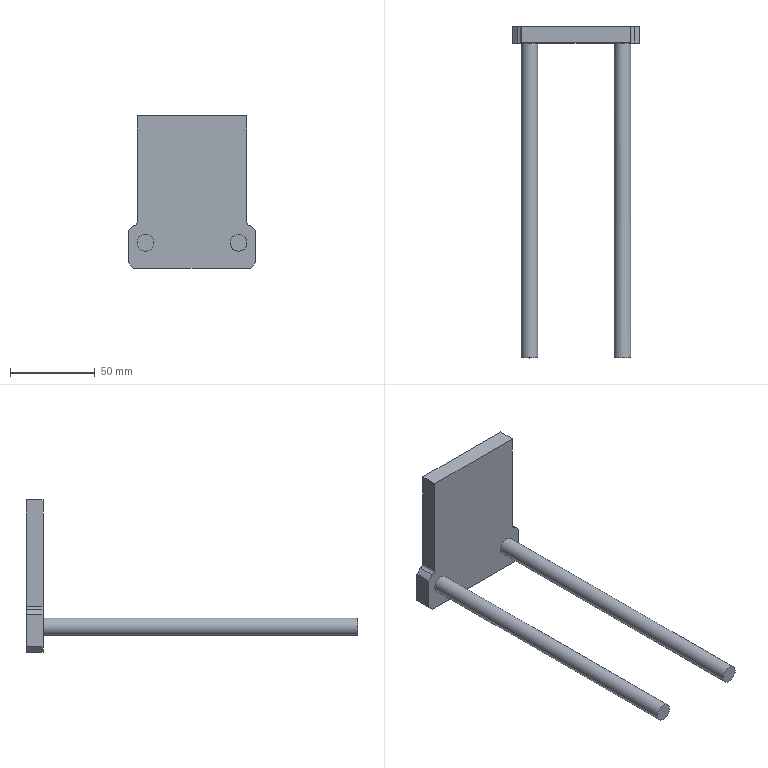Part | STEP file | Tube necking machine_id406_x_t | 1 solid | 18 faces | box 75 x 196.3 x 90 mm | volume 90101 mm3 | plane 14 | cylinder 4 | commonest cylinder face diameters 4 x2 10 x2
STEP:
#1=CARTESIAN_POINT('',(0.,0.,0.));
#2=DIRECTION('',(0.,0.,1.));
#3=DIRECTION('',(1.,0.,0.));
#4=AXIS2_PLACEMENT_3D('',#1,#2,#3);
#5=CARTESIAN_POINT('',(-32.452,292.8,213.016));
#6=VERTEX_POINT('',#5);
#7=CARTESIAN_POINT('',(-32.452,292.8,276.016));
#8=VERTEX_POINT('',#7);
#9=CARTESIAN_POINT('',(-32.452,292.8,186.016));
#10=DIRECTION('',(0.,0.,1.));
#11=VECTOR('',#10,1.);
#12=LINE('',#9,#11);
#13=CARTESIAN_POINT('',(-32.452,292.8,186.016));
#14=DIRECTION('',(1.,0.,0.));
#15=DIRECTION('',(0.,0.,-1.));
#16=AXIS2_PLACEMENT_3D('',#13,#14,#15);
#17=PLANE('',#16);
#18=CARTESIAN_POINT('',(0.,0.));
#19=DIRECTION('',(-1.,0.));
#20=VECTOR('',#19,1.);
#21=LINE('',#18,#20);
#22=(GEOMETRIC_REPRESENTATION_CONTEXT(2)PARAMETRIC_REPRESENTATION_CONTEXT()REPRESENTATION_CONTEXT('',''));
#23=DEFINITIONAL_REPRESENTATION('',(#21),#22);
#24=PCURVE('',#17,#23);
#25=CARTESIAN_POINT('',(0.,292.8,25.));
#26=DIRECTION('',(0.,1.,0.));
#27=DIRECTION('',(0.,0.,1.));
#28=AXIS2_PLACEMENT_3D('',#25,#26,#27);
#29=PLANE('',#28);
#30=CARTESIAN_POINT('',(161.016,-32.452));
#31=DIRECTION('',(1.,0.));
#32=VECTOR('',#31,1.);
#33=LINE('',#30,#32);
#34=(GEOMETRIC_REPRESENTATION_CONTEXT(2)PARAMETRIC_REPRESENTATION_CONTEXT()REPRESENTATION_CONTEXT('',''));
#35=DEFINITIONAL_REPRESENTATION('',(#33),#34);
#36=PCURVE('',#29,#35);
#37=SURFACE_CURVE('',#12,(#24,#36),.PCURVE_S1.);
#38=EDGE_CURVE('',#6,#8,#37,.T.);
#39=ORIENTED_EDGE('',*,*,#38,.F.);
#40=CARTESIAN_POINT('',(-32.452,282.8,213.016));
#41=VERTEX_POINT('',#40);
#42=CARTESIAN_POINT('',(-32.452,292.8,213.016));
#43=DIRECTION('',(0.,-1.,0.));
#44=VECTOR('',#43,1.);
#45=LINE('',#42,#44);
#46=CARTESIAN_POINT('',(-27.,0.));
#47=DIRECTION('',(0.,-1.));
#48=VECTOR('',#47,1.);
#49=LINE('',#46,#48);
#50=(GEOMETRIC_REPRESENTATION_CONTEXT(2)PARAMETRIC_REPRESENTATION_CONTEXT()REPRESENTATION_CONTEXT('',''));
#51=DEFINITIONAL_REPRESENTATION('',(#49),#50);
#52=PCURVE('',#17,#51);
#53=CARTESIAN_POINT('',(-34.452,282.8,213.016));
#54=DIRECTION('',(0.,1.,0.));
#55=DIRECTION('',(0.,0.,1.));
#56=AXIS2_PLACEMENT_3D('',#53,#54,#55);
#57=CYLINDRICAL_SURFACE('',#56,2.);
#58=CARTESIAN_POINT('',(1.571,10.));
#59=DIRECTION('',(0.,-1.));
#60=VECTOR('',#59,1.);
#61=LINE('',#58,#60);
#62=(GEOMETRIC_REPRESENTATION_CONTEXT(2)PARAMETRIC_REPRESENTATION_CONTEXT()REPRESENTATION_CONTEXT('',''));
#63=DEFINITIONAL_REPRESENTATION('',(#61),#62);
#64=PCURVE('',#57,#63);
#65=SURFACE_CURVE('',#45,(#52,#64),.PCURVE_S1.);
#66=EDGE_CURVE('',#6,#41,#65,.T.);
#67=ORIENTED_EDGE('',*,*,#66,.T.);
#68=CARTESIAN_POINT('',(-32.452,282.8,276.016));
#69=VERTEX_POINT('',#68);
#70=CARTESIAN_POINT('',(-32.452,282.8,186.016));
#71=DIRECTION('',(0.,0.,1.));
#72=VECTOR('',#71,1.);
#73=LINE('',#70,#72);
#74=CARTESIAN_POINT('',(0.,-10.));
#75=DIRECTION('',(-1.,0.));
#76=VECTOR('',#75,1.);
#77=LINE('',#74,#76);
#78=(GEOMETRIC_REPRESENTATION_CONTEXT(2)PARAMETRIC_REPRESENTATION_CONTEXT()REPRESENTATION_CONTEXT('',''));
#79=DEFINITIONAL_REPRESENTATION('',(#77),#78);
#80=PCURVE('',#17,#79);
#81=CARTESIAN_POINT('',(0.,282.8,25.));
#82=DIRECTION('',(0.,1.,0.));
#83=DIRECTION('',(0.,0.,1.));
#84=AXIS2_PLACEMENT_3D('',#81,#82,#83);
#85=PLANE('',#84);
#86=CARTESIAN_POINT('',(161.016,-32.452));
#87=DIRECTION('',(1.,0.));
#88=VECTOR('',#87,1.);
#89=LINE('',#86,#88);
#90=(GEOMETRIC_REPRESENTATION_CONTEXT(2)PARAMETRIC_REPRESENTATION_CONTEXT()REPRESENTATION_CONTEXT('',''));
#91=DEFINITIONAL_REPRESENTATION('',(#89),#90);
#92=PCURVE('',#85,#91);
#93=SURFACE_CURVE('',#73,(#80,#92),.PCURVE_S1.);
#94=EDGE_CURVE('',#41,#69,#93,.T.);
#95=ORIENTED_EDGE('',*,*,#94,.T.);
#96=CARTESIAN_POINT('',(-32.452,292.8,276.016));
#97=DIRECTION('',(0.,-1.,0.));
#98=VECTOR('',#97,1.);
#99=LINE('',#96,#98);
#100=CARTESIAN_POINT('',(-90.,0.));
#101=DIRECTION('',(0.,-1.));
#102=VECTOR('',#101,1.);
#103=LINE('',#100,#102);
#104=(GEOMETRIC_REPRESENTATION_CONTEXT(2)PARAMETRIC_REPRESENTATION_CONTEXT()REPRESENTATION_CONTEXT('',''));
#105=DEFINITIONAL_REPRESENTATION('',(#103),#104);
#106=PCURVE('',#17,#105);
#107=CARTESIAN_POINT('',(-32.452,292.8,276.016));
#108=DIRECTION('',(0.,0.,-1.));
#109=DIRECTION('',(-1.,0.,0.));
#110=AXIS2_PLACEMENT_3D('',#107,#108,#109);
#111=PLANE('',#110);
#112=CARTESIAN_POINT('',(0.,0.));
#113=DIRECTION('',(0.,-1.));
#114=VECTOR('',#113,1.);
#115=LINE('',#112,#114);
#116=(GEOMETRIC_REPRESENTATION_CONTEXT(2)PARAMETRIC_REPRESENTATION_CONTEXT()REPRESENTATION_CONTEXT('',''));
#117=DEFINITIONAL_REPRESENTATION('',(#115),#116);
#118=PCURVE('',#111,#117);
#119=SURFACE_CURVE('',#99,(#106,#118),.PCURVE_S1.);
#120=EDGE_CURVE('',#8,#69,#119,.T.);
#121=ORIENTED_EDGE('',*,*,#120,.F.);
#122=EDGE_LOOP('',(#39,#67,#95,#121));
#123=FACE_BOUND('',#122,.T.);
#124=ADVANCED_FACE('',(#123),#17,.F.);
#125=CARTESIAN_POINT('',(32.548,282.8,276.016));
#126=VERTEX_POINT('',#125);
#127=CARTESIAN_POINT('',(-32.452,282.8,276.016));
#128=DIRECTION('',(1.,0.,0.));
#129=VECTOR('',#128,1.);
#130=LINE('',#127,#129);
#131=CARTESIAN_POINT('',(0.,-10.));
#132=DIRECTION('',(-1.,0.));
#133=VECTOR('',#132,1.);
#134=LINE('',#131,#133);
#135=(GEOMETRIC_REPRESENTATION_CONTEXT(2)PARAMETRIC_REPRESENTATION_CONTEXT()REPRESENTATION_CONTEXT('',''));
#136=DEFINITIONAL_REPRESENTATION('',(#134),#135);
#137=PCURVE('',#111,#136);
#138=CARTESIAN_POINT('',(251.016,-32.452));
#139=DIRECTION('',(0.,1.));
#140=VECTOR('',#139,1.);
#141=LINE('',#138,#140);
#142=(GEOMETRIC_REPRESENTATION_CONTEXT(2)PARAMETRIC_REPRESENTATION_CONTEXT()REPRESENTATION_CONTEXT('',''));
#143=DEFINITIONAL_REPRESENTATION('',(#141),#142);
#144=PCURVE('',#85,#143);
#145=SURFACE_CURVE('',#130,(#137,#144),.PCURVE_S1.);
#146=EDGE_CURVE('',#69,#126,#145,.T.);
#147=ORIENTED_EDGE('',*,*,#146,.T.);
#148=CARTESIAN_POINT('',(32.548,292.8,276.016));
#149=VERTEX_POINT('',#148);
#150=CARTESIAN_POINT('',(32.548,292.8,276.016));
#151=DIRECTION('',(0.,-1.,0.));
#152=VECTOR('',#151,1.);
#153=LINE('',#150,#152);
#154=CARTESIAN_POINT('',(-65.,0.));
#155=DIRECTION('',(0.,-1.));
#156=VECTOR('',#155,1.);
#157=LINE('',#154,#156);
#158=(GEOMETRIC_REPRESENTATION_CONTEXT(2)PARAMETRIC_REPRESENTATION_CONTEXT()REPRESENTATION_CONTEXT('',''));
#159=DEFINITIONAL_REPRESENTATION('',(#157),#158);
#160=PCURVE('',#111,#159);
#161=CARTESIAN_POINT('',(32.548,292.8,276.016));
#162=DIRECTION('',(-1.,0.,0.));
#163=DIRECTION('',(0.,0.,1.));
#164=AXIS2_PLACEMENT_3D('',#161,#162,#163);
#165=PLANE('',#164);
#166=CARTESIAN_POINT('',(0.,0.));
#167=DIRECTION('',(0.,-1.));
#168=VECTOR('',#167,1.);
#169=LINE('',#166,#168);
#170=(GEOMETRIC_REPRESENTATION_CONTEXT(2)PARAMETRIC_REPRESENTATION_CONTEXT()REPRESENTATION_CONTEXT('',''));
#171=DEFINITIONAL_REPRESENTATION('',(#169),#170);
#172=PCURVE('',#165,#171);
#173=SURFACE_CURVE('',#153,(#160,#172),.PCURVE_S1.);
#174=EDGE_CURVE('',#149,#126,#173,.T.);
#175=ORIENTED_EDGE('',*,*,#174,.F.);
#176=CARTESIAN_POINT('',(-32.452,292.8,276.016));
#177=DIRECTION('',(1.,0.,0.));
#178=VECTOR('',#177,1.);
#179=LINE('',#176,#178);
#180=CARTESIAN_POINT('',(0.,0.));
#181=DIRECTION('',(-1.,0.));
#182=VECTOR('',#181,1.);
#183=LINE('',#180,#182);
#184=(GEOMETRIC_REPRESENTATION_CONTEXT(2)PARAMETRIC_REPRESENTATION_CONTEXT()REPRESENTATION_CONTEXT('',''));
#185=DEFINITIONAL_REPRESENTATION('',(#183),#184);
#186=PCURVE('',#111,#185);
#187=CARTESIAN_POINT('',(251.016,-32.452));
#188=DIRECTION('',(0.,1.));
#189=VECTOR('',#188,1.);
#190=LINE('',#187,#189);
#191=(GEOMETRIC_REPRESENTATION_CONTEXT(2)PARAMETRIC_REPRESENTATION_CONTEXT()REPRESENTATION_CONTEXT('',''));
#192=DEFINITIONAL_REPRESENTATION('',(#190),#191);
#193=PCURVE('',#29,#192);
#194=SURFACE_CURVE('',#179,(#186,#193),.PCURVE_S1.);
#195=EDGE_CURVE('',#8,#149,#194,.T.);
#196=ORIENTED_EDGE('',*,*,#195,.F.);
#197=ORIENTED_EDGE('',*,*,#120,.T.);
#198=EDGE_LOOP('',(#147,#175,#196,#197));
#199=FACE_BOUND('',#198,.T.);
#200=ADVANCED_FACE('',(#199),#111,.F.);
#201=CARTESIAN_POINT('',(32.548,282.8,213.016));
#202=VERTEX_POINT('',#201);
#203=CARTESIAN_POINT('',(32.548,282.8,276.016));
#204=DIRECTION('',(0.,0.,-1.));
#205=VECTOR('',#204,1.);
#206=LINE('',#203,#205);
#207=CARTESIAN_POINT('',(0.,-10.));
#208=DIRECTION('',(-1.,0.));
#209=VECTOR('',#208,1.);
#210=LINE('',#207,#209);
#211=(GEOMETRIC_REPRESENTATION_CONTEXT(2)PARAMETRIC_REPRESENTATION_CONTEXT()REPRESENTATION_CONTEXT('',''));
#212=DEFINITIONAL_REPRESENTATION('',(#210),#211);
#213=PCURVE('',#165,#212);
#214=CARTESIAN_POINT('',(251.016,32.548));
#215=DIRECTION('',(-1.,0.));
#216=VECTOR('',#215,1.);
#217=LINE('',#214,#216);
#218=(GEOMETRIC_REPRESENTATION_CONTEXT(2)PARAMETRIC_REPRESENTATION_CONTEXT()REPRESENTATION_CONTEXT('',''));
#219=DEFINITIONAL_REPRESENTATION('',(#217),#218);
#220=PCURVE('',#85,#219);
#221=SURFACE_CURVE('',#206,(#213,#220),.PCURVE_S1.);
#222=EDGE_CURVE('',#126,#202,#221,.T.);
#223=ORIENTED_EDGE('',*,*,#222,.T.);
#224=CARTESIAN_POINT('',(32.548,292.8,213.016));
#225=VERTEX_POINT('',#224);
#226=CARTESIAN_POINT('',(32.548,292.8,213.016));
#227=DIRECTION('',(0.,1.,0.));
#228=VECTOR('',#227,1.);
#229=LINE('',#226,#228);
#230=CARTESIAN_POINT('',(-63.,0.));
#231=DIRECTION('',(0.,1.));
#232=VECTOR('',#231,1.);
#233=LINE('',#230,#232);
#234=(GEOMETRIC_REPRESENTATION_CONTEXT(2)PARAMETRIC_REPRESENTATION_CONTEXT()REPRESENTATION_CONTEXT('',''));
#235=DEFINITIONAL_REPRESENTATION('',(#233),#234);
#236=PCURVE('',#165,#235);
#237=CARTESIAN_POINT('',(34.548,292.8,213.016));
#238=DIRECTION('',(0.,-1.,0.));
#239=DIRECTION('',(0.,0.,-1.));
#240=AXIS2_PLACEMENT_3D('',#237,#238,#239);
#241=CYLINDRICAL_SURFACE('',#240,2.);
#242=CARTESIAN_POINT('',(4.712,0.));
#243=DIRECTION('',(0.,-1.));
#244=VECTOR('',#243,1.);
#245=LINE('',#242,#244);
#246=(GEOMETRIC_REPRESENTATION_CONTEXT(2)PARAMETRIC_REPRESENTATION_CONTEXT()REPRESENTATION_CONTEXT('',''));
#247=DEFINITIONAL_REPRESENTATION('',(#245),#246);
#248=PCURVE('',#241,#247);
#249=SURFACE_CURVE('',#229,(#236,#248),.PCURVE_S1.);
#250=EDGE_CURVE('',#202,#225,#249,.T.);
#251=ORIENTED_EDGE('',*,*,#250,.T.);
#252=CARTESIAN_POINT('',(32.548,292.8,276.016));
#253=DIRECTION('',(0.,0.,-1.));
#254=VECTOR('',#253,1.);
#255=LINE('',#252,#254);
#256=CARTESIAN_POINT('',(0.,0.));
#257=DIRECTION('',(-1.,0.));
#258=VECTOR('',#257,1.);
#259=LINE('',#256,#258);
#260=(GEOMETRIC_REPRESENTATION_CONTEXT(2)PARAMETRIC_REPRESENTATION_CONTEXT()REPRESENTATION_CONTEXT('',''));
#261=DEFINITIONAL_REPRESENTATION('',(#259),#260);
#262=PCURVE('',#165,#261);
#263=CARTESIAN_POINT('',(251.016,32.548));
#264=DIRECTION('',(-1.,0.));
#265=VECTOR('',#264,1.);
#266=LINE('',#263,#265);
#267=(GEOMETRIC_REPRESENTATION_CONTEXT(2)PARAMETRIC_REPRESENTATION_CONTEXT()REPRESENTATION_CONTEXT('',''));
#268=DEFINITIONAL_REPRESENTATION('',(#266),#267);
#269=PCURVE('',#29,#268);
#270=SURFACE_CURVE('',#255,(#262,#269),.PCURVE_S1.);
#271=EDGE_CURVE('',#149,#225,#270,.T.);
#272=ORIENTED_EDGE('',*,*,#271,.F.);
#273=ORIENTED_EDGE('',*,*,#174,.T.);
#274=EDGE_LOOP('',(#223,#251,#272,#273));
#275=FACE_BOUND('',#274,.T.);
#276=ADVANCED_FACE('',(#275),#165,.F.);
#277=CARTESIAN_POINT('',(34.548,292.8,186.016));
#278=VERTEX_POINT('',#277);
#279=CARTESIAN_POINT('',(-34.452,292.8,186.016));
#280=VERTEX_POINT('',#279);
#281=CARTESIAN_POINT('',(32.548,292.8,186.016));
#282=DIRECTION('',(-1.,0.,0.));
#283=VECTOR('',#282,1.);
#284=LINE('',#281,#283);
#285=CARTESIAN_POINT('',(32.548,292.8,186.016));
#286=DIRECTION('',(0.,0.,1.));
#287=DIRECTION('',(1.,0.,0.));
#288=AXIS2_PLACEMENT_3D('',#285,#286,#287);
#289=PLANE('',#288);
#290=CARTESIAN_POINT('',(0.,0.));
#291=DIRECTION('',(-1.,0.));
#292=VECTOR('',#291,1.);
#293=LINE('',#290,#292);
#294=(GEOMETRIC_REPRESENTATION_CONTEXT(2)PARAMETRIC_REPRESENTATION_CONTEXT()REPRESENTATION_CONTEXT('',''));
#295=DEFINITIONAL_REPRESENTATION('',(#293),#294);
#296=PCURVE('',#289,#295);
#297=CARTESIAN_POINT('',(161.016,32.548));
#298=DIRECTION('',(0.,-1.));
#299=VECTOR('',#298,1.);
#300=LINE('',#297,#299);
#301=(GEOMETRIC_REPRESENTATION_CONTEXT(2)PARAMETRIC_REPRESENTATION_CONTEXT()REPRESENTATION_CONTEXT('',''));
#302=DEFINITIONAL_REPRESENTATION('',(#300),#301);
#303=PCURVE('',#29,#302);
#304=SURFACE_CURVE('',#284,(#296,#303),.PCURVE_S1.);
#305=EDGE_CURVE('',#278,#280,#304,.T.);
#306=ORIENTED_EDGE('',*,*,#305,.F.);
#307=CARTESIAN_POINT('',(34.548,282.8,186.016));
#308=VERTEX_POINT('',#307);
#309=CARTESIAN_POINT('',(34.548,292.8,186.016));
#310=DIRECTION('',(0.,-1.,0.));
#311=VECTOR('',#310,1.);
#312=LINE('',#309,#311);
#313=CARTESIAN_POINT('',(2.,0.));
#314=DIRECTION('',(0.,-1.));
#315=VECTOR('',#314,1.);
#316=LINE('',#313,#315);
#317=(GEOMETRIC_REPRESENTATION_CONTEXT(2)PARAMETRIC_REPRESENTATION_CONTEXT()REPRESENTATION_CONTEXT('',''));
#318=DEFINITIONAL_REPRESENTATION('',(#316),#317);
#319=PCURVE('',#289,#318);
#320=CARTESIAN_POINT('',(37.548,282.8,189.016));
#321=DIRECTION('',(-0.7071,0.,0.7071));
#322=DIRECTION('',(0.,1.,0.));
#323=AXIS2_PLACEMENT_3D('',#320,#321,#322);
#324=PLANE('',#323);
#325=CARTESIAN_POINT('',(10.,4.243));
#326=DIRECTION('',(-1.,0.));
#327=VECTOR('',#326,1.);
#328=LINE('',#325,#327);
#329=(GEOMETRIC_REPRESENTATION_CONTEXT(2)PARAMETRIC_REPRESENTATION_CONTEXT()REPRESENTATION_CONTEXT('',''));
#330=DEFINITIONAL_REPRESENTATION('',(#328),#329);
#331=PCURVE('',#324,#330);
#332=SURFACE_CURVE('',#312,(#319,#331),.PCURVE_S1.);
#333=EDGE_CURVE('',#278,#308,#332,.T.);
#334=ORIENTED_EDGE('',*,*,#333,.T.);
#335=CARTESIAN_POINT('',(-34.452,282.8,186.016));
#336=VERTEX_POINT('',#335);
#337=CARTESIAN_POINT('',(32.548,282.8,186.016));
#338=DIRECTION('',(-1.,0.,0.));
#339=VECTOR('',#338,1.);
#340=LINE('',#337,#339);
#341=CARTESIAN_POINT('',(0.,-10.));
#342=DIRECTION('',(-1.,0.));
#343=VECTOR('',#342,1.);
#344=LINE('',#341,#343);
#345=(GEOMETRIC_REPRESENTATION_CONTEXT(2)PARAMETRIC_REPRESENTATION_CONTEXT()REPRESENTATION_CONTEXT('',''));
#346=DEFINITIONAL_REPRESENTATION('',(#344),#345);
#347=PCURVE('',#289,#346);
#348=CARTESIAN_POINT('',(161.016,32.548));
#349=DIRECTION('',(0.,-1.));
#350=VECTOR('',#349,1.);
#351=LINE('',#348,#350);
#352=(GEOMETRIC_REPRESENTATION_CONTEXT(2)PARAMETRIC_REPRESENTATION_CONTEXT()REPRESENTATION_CONTEXT('',''));
#353=DEFINITIONAL_REPRESENTATION('',(#351),#352);
#354=PCURVE('',#85,#353);
#355=SURFACE_CURVE('',#340,(#347,#354),.PCURVE_S1.);
#356=EDGE_CURVE('',#308,#336,#355,.T.);
#357=ORIENTED_EDGE('',*,*,#356,.T.);
#358=CARTESIAN_POINT('',(-34.452,292.8,186.016));
#359=DIRECTION('',(0.,1.,0.));
#360=VECTOR('',#359,1.);
#361=LINE('',#358,#360);
#362=CARTESIAN_POINT('',(-67.,0.));
#363=DIRECTION('',(0.,1.));
#364=VECTOR('',#363,1.);
#365=LINE('',#362,#364);
#366=(GEOMETRIC_REPRESENTATION_CONTEXT(2)PARAMETRIC_REPRESENTATION_CONTEXT()REPRESENTATION_CONTEXT('',''));
#367=DEFINITIONAL_REPRESENTATION('',(#365),#366);
#368=PCURVE('',#289,#367);
#369=CARTESIAN_POINT('',(-34.452,292.8,186.016));
#370=DIRECTION('',(-0.7071,0.,-0.7071));
#371=DIRECTION('',(0.,-1.,0.));
#372=AXIS2_PLACEMENT_3D('',#369,#370,#371);
#373=PLANE('',#372);
#374=CARTESIAN_POINT('',(0.,0.));
#375=DIRECTION('',(-1.,0.));
#376=VECTOR('',#375,1.);
#377=LINE('',#374,#376);
#378=(GEOMETRIC_REPRESENTATION_CONTEXT(2)PARAMETRIC_REPRESENTATION_CONTEXT()REPRESENTATION_CONTEXT('',''));
#379=DEFINITIONAL_REPRESENTATION('',(#377),#378);
#380=PCURVE('',#373,#379);
#381=SURFACE_CURVE('',#361,(#368,#380),.PCURVE_S1.);
#382=EDGE_CURVE('',#336,#280,#381,.T.);
#383=ORIENTED_EDGE('',*,*,#382,.T.);
#384=EDGE_LOOP('',(#306,#334,#357,#383));
#385=FACE_BOUND('',#384,.T.);
#386=ADVANCED_FACE('',(#385),#289,.F.);
#387=CARTESIAN_POINT('',(34.548,292.8,211.016));
#388=VERTEX_POINT('',#387);
#389=CARTESIAN_POINT('',(34.548,292.8,213.016));
#390=DIRECTION('',(0.,-1.,0.));
#391=DIRECTION('',(0.,0.,1.));
#392=AXIS2_PLACEMENT_3D('',#389,#390,#391);
#393=CIRCLE('',#392,2.);
#394=CARTESIAN_POINT('',(190.016,34.548));
#395=CARTESIAN_POINT('',(190.016,31.084));
#396=CARTESIAN_POINT('',(187.016,32.816));
#397=CARTESIAN_POINT('',(184.016,34.548));
#398=CARTESIAN_POINT('',(187.016,36.28));
#399=CARTESIAN_POINT('',(190.016,38.012));
#400=CARTESIAN_POINT('',(190.016,34.548));
#401=(BOUNDED_CURVE()B_SPLINE_CURVE(2,(#394,#395,#396,#397,#398,#399,#400),.UNSPECIFIED.,.T.,.F.)B_SPLINE_CURVE_WITH_KNOTS((1,2,2,2,2,1),(-2.094,0.,2.094,4.189,6.283,8.378),.UNSPECIFIED.)CURVE()GEOMETRIC_REPRESENTATION_ITEM()RATIONAL_B_SPLINE_CURVE((1.,0.5,1.,0.5,1.,0.5,1.))REPRESENTATION_ITEM(''));
#402=(GEOMETRIC_REPRESENTATION_CONTEXT(2)PARAMETRIC_REPRESENTATION_CONTEXT()REPRESENTATION_CONTEXT('',''));
#403=DEFINITIONAL_REPRESENTATION('',(#401),#402);
#404=PCURVE('',#29,#403);
#405=CARTESIAN_POINT('',(3.142,0.));
#406=DIRECTION('',(1.,0.));
#407=VECTOR('',#406,1.);
#408=LINE('',#405,#407);
#409=(GEOMETRIC_REPRESENTATION_CONTEXT(2)PARAMETRIC_REPRESENTATION_CONTEXT()REPRESENTATION_CONTEXT('',''));
#410=DEFINITIONAL_REPRESENTATION('',(#408),#409);
#411=PCURVE('',#241,#410);
#412=SURFACE_CURVE('',#393,(#404,#411),.PCURVE_S1.);
#413=EDGE_CURVE('',#225,#388,#412,.T.);
#414=ORIENTED_EDGE('',*,*,#413,.T.);
#415=CARTESIAN_POINT('',(37.548,292.8,208.016));
#416=VERTEX_POINT('',#415);
#417=CARTESIAN_POINT('',(110.282,292.8,135.282));
#418=DIRECTION('',(0.7071,0.,-0.7071));
#419=VECTOR('',#418,1.);
#420=LINE('',#417,#419);
#421=CARTESIAN_POINT('',(110.282,110.282));
#422=DIRECTION('',(-0.7071,0.7071));
#423=VECTOR('',#422,1.);
#424=LINE('',#421,#423);
#425=(GEOMETRIC_REPRESENTATION_CONTEXT(2)PARAMETRIC_REPRESENTATION_CONTEXT()REPRESENTATION_CONTEXT('',''));
#426=DEFINITIONAL_REPRESENTATION('',(#424),#425);
#427=PCURVE('',#29,#426);
#428=CARTESIAN_POINT('',(34.548,282.8,211.016));
#429=DIRECTION('',(-0.7071,0.,-0.7071));
#430=DIRECTION('',(0.,1.,0.));
#431=AXIS2_PLACEMENT_3D('',#428,#429,#430);
#432=PLANE('',#431);
#433=CARTESIAN_POINT('',(10.,107.104));
#434=DIRECTION('',(0.,1.));
#435=VECTOR('',#434,1.);
#436=LINE('',#433,#435);
#437=(GEOMETRIC_REPRESENTATION_CONTEXT(2)PARAMETRIC_REPRESENTATION_CONTEXT()REPRESENTATION_CONTEXT('',''));
#438=DEFINITIONAL_REPRESENTATION('',(#436),#437);
#439=PCURVE('',#432,#438);
#440=SURFACE_CURVE('',#420,(#427,#439),.PCURVE_S1.);
#441=EDGE_CURVE('',#388,#416,#440,.T.);
#442=ORIENTED_EDGE('',*,*,#441,.T.);
#443=CARTESIAN_POINT('',(37.548,292.8,189.016));
#444=VERTEX_POINT('',#443);
#445=CARTESIAN_POINT('',(37.548,292.8,186.016));
#446=DIRECTION('',(0.,0.,1.));
#447=VECTOR('',#446,1.);
#448=LINE('',#445,#447);
#449=CARTESIAN_POINT('',(161.016,37.548));
#450=DIRECTION('',(1.,0.));
#451=VECTOR('',#450,1.);
#452=LINE('',#449,#451);
#453=(GEOMETRIC_REPRESENTATION_CONTEXT(2)PARAMETRIC_REPRESENTATION_CONTEXT()REPRESENTATION_CONTEXT('',''));
#454=DEFINITIONAL_REPRESENTATION('',(#452),#453);
#455=PCURVE('',#29,#454);
#456=CARTESIAN_POINT('',(37.548,282.8,186.016));
#457=DIRECTION('',(-1.,0.,0.));
#458=DIRECTION('',(0.,0.,1.));
#459=AXIS2_PLACEMENT_3D('',#456,#457,#458);
#460=PLANE('',#459);
#461=CARTESIAN_POINT('',(0.,10.));
#462=DIRECTION('',(1.,0.));
#463=VECTOR('',#462,1.);
#464=LINE('',#461,#463);
#465=(GEOMETRIC_REPRESENTATION_CONTEXT(2)PARAMETRIC_REPRESENTATION_CONTEXT()REPRESENTATION_CONTEXT('',''));
#466=DEFINITIONAL_REPRESENTATION('',(#464),#465);
#467=PCURVE('',#460,#466);
#468=SURFACE_CURVE('',#448,(#455,#467),.PCURVE_S1.);
#469=EDGE_CURVE('',#444,#416,#468,.T.);
#470=ORIENTED_EDGE('',*,*,#469,.F.);
#471=CARTESIAN_POINT('',(-63.234,292.8,88.234));
#472=DIRECTION('',(-0.7071,0.,-0.7071));
#473=VECTOR('',#472,1.);
#474=LINE('',#471,#473);
#475=CARTESIAN_POINT('',(63.234,-63.234));
#476=DIRECTION('',(-0.7071,-0.7071));
#477=VECTOR('',#476,1.);
#478=LINE('',#475,#477);
#479=(GEOMETRIC_REPRESENTATION_CONTEXT(2)PARAMETRIC_REPRESENTATION_CONTEXT()REPRESENTATION_CONTEXT('',''));
#480=DEFINITIONAL_REPRESENTATION('',(#478),#479);
#481=PCURVE('',#29,#480);
#482=CARTESIAN_POINT('',(10.,142.527));
#483=DIRECTION('',(0.,1.));
#484=VECTOR('',#483,1.);
#485=LINE('',#482,#484);
#486=(GEOMETRIC_REPRESENTATION_CONTEXT(2)PARAMETRIC_REPRESENTATION_CONTEXT()REPRESENTATION_CONTEXT('',''));
#487=DEFINITIONAL_REPRESENTATION('',(#485),#486);
#488=PCURVE('',#324,#487);
#489=SURFACE_CURVE('',#474,(#481,#488),.PCURVE_S1.);
#490=EDGE_CURVE('',#444,#278,#489,.T.);
#491=ORIENTED_EDGE('',*,*,#490,.T.);
#492=ORIENTED_EDGE('',*,*,#305,.T.);
#493=CARTESIAN_POINT('',(-37.452,292.8,189.016));
#494=VERTEX_POINT('',#493);
#495=CARTESIAN_POINT('',(63.282,292.8,88.282));
#496=DIRECTION('',(-0.7071,0.,0.7071));
#497=VECTOR('',#496,1.);
#498=LINE('',#495,#497);
#499=CARTESIAN_POINT('',(63.282,63.282));
#500=DIRECTION('',(0.7071,-0.7071));
#501=VECTOR('',#500,1.);
#502=LINE('',#499,#501);
#503=(GEOMETRIC_REPRESENTATION_CONTEXT(2)PARAMETRIC_REPRESENTATION_CONTEXT()REPRESENTATION_CONTEXT('',''));
#504=DEFINITIONAL_REPRESENTATION('',(#502),#503);
#505=PCURVE('',#29,#504);
#506=CARTESIAN_POINT('',(0.,-138.217));
#507=DIRECTION('',(0.,1.));
#508=VECTOR('',#507,1.);
#509=LINE('',#506,#508);
#510=(GEOMETRIC_REPRESENTATION_CONTEXT(2)PARAMETRIC_REPRESENTATION_CONTEXT()REPRESENTATION_CONTEXT('',''));
#511=DEFINITIONAL_REPRESENTATION('',(#509),#510);
#512=PCURVE('',#373,#511);
#513=SURFACE_CURVE('',#498,(#505,#512),.PCURVE_S1.);
#514=EDGE_CURVE('',#280,#494,#513,.T.);
#515=ORIENTED_EDGE('',*,*,#514,.T.);
#516=CARTESIAN_POINT('',(-37.452,292.8,208.016));
#517=VERTEX_POINT('',#516);
#518=CARTESIAN_POINT('',(-37.452,292.8,186.016));
#519=DIRECTION('',(0.,0.,1.));
#520=VECTOR('',#519,1.);
#521=LINE('',#518,#520);
#522=CARTESIAN_POINT('',(161.016,-37.452));
#523=DIRECTION('',(1.,0.));
#524=VECTOR('',#523,1.);
#525=LINE('',#522,#524);
#526=(GEOMETRIC_REPRESENTATION_CONTEXT(2)PARAMETRIC_REPRESENTATION_CONTEXT()REPRESENTATION_CONTEXT('',''));
#527=DEFINITIONAL_REPRESENTATION('',(#525),#526);
#528=PCURVE('',#29,#527);
#529=CARTESIAN_POINT('',(-37.452,282.8,186.016));
#530=DIRECTION('',(-1.,0.,0.));
#531=DIRECTION('',(0.,0.,1.));
#532=AXIS2_PLACEMENT_3D('',#529,#530,#531);
#533=PLANE('',#532);
#534=CARTESIAN_POINT('',(0.,10.));
#535=DIRECTION('',(1.,0.));
#536=VECTOR('',#535,1.);
#537=LINE('',#534,#536);
#538=(GEOMETRIC_REPRESENTATION_CONTEXT(2)PARAMETRIC_REPRESENTATION_CONTEXT()REPRESENTATION_CONTEXT('',''));
#539=DEFINITIONAL_REPRESENTATION('',(#537),#538);
#540=PCURVE('',#533,#539);
#541=SURFACE_CURVE('',#521,(#528,#540),.PCURVE_S1.);
#542=EDGE_CURVE('',#494,#517,#541,.T.);
#543=ORIENTED_EDGE('',*,*,#542,.T.);
#544=CARTESIAN_POINT('',(-34.452,292.8,211.016));
#545=VERTEX_POINT('',#544);
#546=CARTESIAN_POINT('',(-110.234,292.8,135.234));
#547=DIRECTION('',(0.7071,0.,0.7071));
#548=VECTOR('',#547,1.);
#549=LINE('',#546,#548);
#550=CARTESIAN_POINT('',(110.234,-110.234));
#551=DIRECTION('',(0.7071,0.7071));
#552=VECTOR('',#551,1.);
#553=LINE('',#550,#552);
#554=(GEOMETRIC_REPRESENTATION_CONTEXT(2)PARAMETRIC_REPRESENTATION_CONTEXT()REPRESENTATION_CONTEXT('',''));
#555=DEFINITIONAL_REPRESENTATION('',(#553),#554);
#556=PCURVE('',#29,#555);
#557=CARTESIAN_POINT('',(-37.452,282.8,208.016));
#558=DIRECTION('',(0.7071,0.,-0.7071));
#559=DIRECTION('',(0.,1.,0.));
#560=AXIS2_PLACEMENT_3D('',#557,#558,#559);
#561=PLANE('',#560);
#562=CARTESIAN_POINT('',(10.,-102.929));
#563=DIRECTION('',(0.,1.));
#564=VECTOR('',#563,1.);
#565=LINE('',#562,#564);
#566=(GEOMETRIC_REPRESENTATION_CONTEXT(2)PARAMETRIC_REPRESENTATION_CONTEXT()REPRESENTATION_CONTEXT('',''));
#567=DEFINITIONAL_REPRESENTATION('',(#565),#566);
#568=PCURVE('',#561,#567);
#569=SURFACE_CURVE('',#549,(#556,#568),.PCURVE_S1.);
#570=EDGE_CURVE('',#517,#545,#569,.T.);
#571=ORIENTED_EDGE('',*,*,#570,.T.);
#572=CARTESIAN_POINT('',(-34.452,292.8,213.016));
#573=DIRECTION('',(0.,-1.,0.));
#574=DIRECTION('',(0.,0.,1.));
#575=AXIS2_PLACEMENT_3D('',#572,#573,#574);
#576=CIRCLE('',#575,2.);
#577=CARTESIAN_POINT('',(190.016,-34.452));
#578=CARTESIAN_POINT('',(190.016,-37.916));
#579=CARTESIAN_POINT('',(187.016,-36.184));
#580=CARTESIAN_POINT('',(184.016,-34.452));
#581=CARTESIAN_POINT('',(187.016,-32.72));
#582=CARTESIAN_POINT('',(190.016,-30.988));
#583=CARTESIAN_POINT('',(190.016,-34.452));
#584=(BOUNDED_CURVE()B_SPLINE_CURVE(2,(#577,#578,#579,#580,#581,#582,#583),.UNSPECIFIED.,.T.,.F.)B_SPLINE_CURVE_WITH_KNOTS((1,2,2,2,2,1),(-2.094,0.,2.094,4.189,6.283,8.378),.UNSPECIFIED.)CURVE()GEOMETRIC_REPRESENTATION_ITEM()RATIONAL_B_SPLINE_CURVE((1.,0.5,1.,0.5,1.,0.5,1.))REPRESENTATION_ITEM(''));
#585=(GEOMETRIC_REPRESENTATION_CONTEXT(2)PARAMETRIC_REPRESENTATION_CONTEXT()REPRESENTATION_CONTEXT('',''));
#586=DEFINITIONAL_REPRESENTATION('',(#584),#585);
#587=PCURVE('',#29,#586);
#588=CARTESIAN_POINT('',(6.283,10.));
#589=DIRECTION('',(-1.,0.));
#590=VECTOR('',#589,1.);
#591=LINE('',#588,#590);
#592=(GEOMETRIC_REPRESENTATION_CONTEXT(2)PARAMETRIC_REPRESENTATION_CONTEXT()REPRESENTATION_CONTEXT('',''));
#593=DEFINITIONAL_REPRESENTATION('',(#591),#592);
#594=PCURVE('',#57,#593);
#595=SURFACE_CURVE('',#576,(#587,#594),.PCURVE_S1.);
#596=EDGE_CURVE('',#545,#6,#595,.T.);
#597=ORIENTED_EDGE('',*,*,#596,.T.);
#598=ORIENTED_EDGE('',*,*,#38,.T.);
#599=ORIENTED_EDGE('',*,*,#195,.T.);
#600=ORIENTED_EDGE('',*,*,#271,.T.);
#601=EDGE_LOOP('',(#414,#442,#470,#491,#492,#515,#543,#571,#597,#598,#599,#600));
#602=FACE_BOUND('',#601,.T.);
#603=ADVANCED_FACE('',(#602),#29,.T.);
#604=CARTESIAN_POINT('',(27.548,282.8,206.016));
#605=VERTEX_POINT('',#604);
#606=CARTESIAN_POINT('',(27.548,282.8,201.016));
#607=DIRECTION('',(0.,1.,0.));
#608=DIRECTION('',(0.,0.,1.));
#609=AXIS2_PLACEMENT_3D('',#606,#607,#608);
#610=CIRCLE('',#609,5.);
#611=CARTESIAN_POINT('',(176.016,27.548));
#612=DIRECTION('',(1.,0.));
#613=AXIS2_PLACEMENT_2D('',#611,#612);
#614=CIRCLE('',#613,5.);
#615=(GEOMETRIC_REPRESENTATION_CONTEXT(2)PARAMETRIC_REPRESENTATION_CONTEXT()REPRESENTATION_CONTEXT('',''));
#616=DEFINITIONAL_REPRESENTATION('',(#614),#615);
#617=PCURVE('',#85,#616);
#618=CARTESIAN_POINT('',(27.548,172.8,201.016));
#619=DIRECTION('',(0.,1.,0.));
#620=DIRECTION('',(0.,0.,1.));
#621=AXIS2_PLACEMENT_3D('',#618,#619,#620);
#622=CYLINDRICAL_SURFACE('',#621,5.);
#623=CARTESIAN_POINT('',(0.,110.));
#624=DIRECTION('',(1.,0.));
#625=VECTOR('',#624,1.);
#626=LINE('',#623,#625);
#627=(GEOMETRIC_REPRESENTATION_CONTEXT(2)PARAMETRIC_REPRESENTATION_CONTEXT()REPRESENTATION_CONTEXT('',''));
#628=DEFINITIONAL_REPRESENTATION('',(#626),#627);
#629=PCURVE('',#622,#628);
#630=SURFACE_CURVE('',#610,(#617,#629),.PCURVE_S1.);
#631=EDGE_CURVE('',#605,#605,#630,.T.);
#632=ORIENTED_EDGE('',*,*,#631,.T.);
#633=EDGE_LOOP('',(#632));
#634=FACE_BOUND('',#633,.T.);
#635=CARTESIAN_POINT('',(-27.452,282.8,206.016));
#636=VERTEX_POINT('',#635);
#637=CARTESIAN_POINT('',(-27.452,282.8,201.016));
#638=DIRECTION('',(0.,-1.,0.));
#639=DIRECTION('',(0.,0.,1.));
#640=AXIS2_PLACEMENT_3D('',#637,#638,#639);
#641=CIRCLE('',#640,5.);
#642=CARTESIAN_POINT('',(181.016,-27.452));
#643=CARTESIAN_POINT('',(181.016,-36.113));
#644=CARTESIAN_POINT('',(173.516,-31.782));
#645=CARTESIAN_POINT('',(166.016,-27.452));
#646=CARTESIAN_POINT('',(173.516,-23.122));
#647=CARTESIAN_POINT('',(181.016,-18.792));
#648=CARTESIAN_POINT('',(181.016,-27.452));
#649=(BOUNDED_CURVE()B_SPLINE_CURVE(2,(#642,#643,#644,#645,#646,#647,#648),.UNSPECIFIED.,.T.,.F.)B_SPLINE_CURVE_WITH_KNOTS((1,2,2,2,2,1),(-2.094,0.,2.094,4.189,6.283,8.378),.UNSPECIFIED.)CURVE()GEOMETRIC_REPRESENTATION_ITEM()RATIONAL_B_SPLINE_CURVE((1.,0.5,1.,0.5,1.,0.5,1.))REPRESENTATION_ITEM(''));
#650=(GEOMETRIC_REPRESENTATION_CONTEXT(2)PARAMETRIC_REPRESENTATION_CONTEXT()REPRESENTATION_CONTEXT('',''));
#651=DEFINITIONAL_REPRESENTATION('',(#649),#650);
#652=PCURVE('',#85,#651);
#653=CARTESIAN_POINT('',(-27.452,172.8,201.016));
#654=DIRECTION('',(0.,1.,0.));
#655=DIRECTION('',(0.,0.,1.));
#656=AXIS2_PLACEMENT_3D('',#653,#654,#655);
#657=CYLINDRICAL_SURFACE('',#656,5.);
#658=CARTESIAN_POINT('',(6.283,110.));
#659=DIRECTION('',(-1.,0.));
#660=VECTOR('',#659,1.);
#661=LINE('',#658,#660);
#662=(GEOMETRIC_REPRESENTATION_CONTEXT(2)PARAMETRIC_REPRESENTATION_CONTEXT()REPRESENTATION_CONTEXT('',''));
#663=DEFINITIONAL_REPRESENTATION('',(#661),#662);
#664=PCURVE('',#657,#663);
#665=SURFACE_CURVE('',#641,(#652,#664),.PCURVE_S1.);
#666=EDGE_CURVE('',#636,#636,#665,.T.);
#667=ORIENTED_EDGE('',*,*,#666,.F.);
#668=EDGE_LOOP('',(#667));
#669=FACE_BOUND('',#668,.T.);
#670=CARTESIAN_POINT('',(37.548,282.8,189.016));
#671=VERTEX_POINT('',#670);
#672=CARTESIAN_POINT('',(37.548,282.8,208.016));
#673=VERTEX_POINT('',#672);
#674=CARTESIAN_POINT('',(37.548,282.8,186.016));
#675=DIRECTION('',(0.,0.,1.));
#676=VECTOR('',#675,1.);
#677=LINE('',#674,#676);
#678=CARTESIAN_POINT('',(161.016,37.548));
#679=DIRECTION('',(1.,0.));
#680=VECTOR('',#679,1.);
#681=LINE('',#678,#680);
#682=(GEOMETRIC_REPRESENTATION_CONTEXT(2)PARAMETRIC_REPRESENTATION_CONTEXT()REPRESENTATION_CONTEXT('',''));
#683=DEFINITIONAL_REPRESENTATION('',(#681),#682);
#684=PCURVE('',#85,#683);
#685=CARTESIAN_POINT('',(0.,0.));
#686=DIRECTION('',(1.,0.));
#687=VECTOR('',#686,1.);
#688=LINE('',#685,#687);
#689=(GEOMETRIC_REPRESENTATION_CONTEXT(2)PARAMETRIC_REPRESENTATION_CONTEXT()REPRESENTATION_CONTEXT('',''));
#690=DEFINITIONAL_REPRESENTATION('',(#688),#689);
#691=PCURVE('',#460,#690);
#692=SURFACE_CURVE('',#677,(#684,#691),.PCURVE_S1.);
#693=EDGE_CURVE('',#671,#673,#692,.T.);
#694=ORIENTED_EDGE('',*,*,#693,.T.);
#695=CARTESIAN_POINT('',(34.548,282.8,211.016));
#696=VERTEX_POINT('',#695);
#697=CARTESIAN_POINT('',(34.548,282.8,211.016));
#698=DIRECTION('',(-0.7071,0.,0.7071));
#699=VECTOR('',#698,1.);
#700=LINE('',#697,#699);
#701=CARTESIAN_POINT('',(186.016,34.548));
#702=DIRECTION('',(0.7071,-0.7071));
#703=VECTOR('',#702,1.);
#704=LINE('',#701,#703);
#705=(GEOMETRIC_REPRESENTATION_CONTEXT(2)PARAMETRIC_REPRESENTATION_CONTEXT()REPRESENTATION_CONTEXT('',''));
#706=DEFINITIONAL_REPRESENTATION('',(#704),#705);
#707=PCURVE('',#85,#706);
#708=CARTESIAN_POINT('',(0.,0.));
#709=DIRECTION('',(0.,-1.));
#710=VECTOR('',#709,1.);
#711=LINE('',#708,#710);
#712=(GEOMETRIC_REPRESENTATION_CONTEXT(2)PARAMETRIC_REPRESENTATION_CONTEXT()REPRESENTATION_CONTEXT('',''));
#713=DEFINITIONAL_REPRESENTATION('',(#711),#712);
#714=PCURVE('',#432,#713);
#715=SURFACE_CURVE('',#700,(#707,#714),.PCURVE_S1.);
#716=EDGE_CURVE('',#673,#696,#715,.T.);
#717=ORIENTED_EDGE('',*,*,#716,.T.);
#718=CARTESIAN_POINT('',(34.548,282.8,213.016));
#719=DIRECTION('',(0.,1.,0.));
#720=DIRECTION('',(0.,0.,1.));
#721=AXIS2_PLACEMENT_3D('',#718,#719,#720);
#722=CIRCLE('',#721,2.);
#723=CARTESIAN_POINT('',(188.016,34.548));
#724=DIRECTION('',(1.,0.));
#725=AXIS2_PLACEMENT_2D('',#723,#724);
#726=CIRCLE('',#725,2.);
#727=(GEOMETRIC_REPRESENTATION_CONTEXT(2)PARAMETRIC_REPRESENTATION_CONTEXT()REPRESENTATION_CONTEXT('',''));
#728=DEFINITIONAL_REPRESENTATION('',(#726),#727);
#729=PCURVE('',#85,#728);
#730=CARTESIAN_POINT('',(9.425,10.));
#731=DIRECTION('',(-1.,0.));
#732=VECTOR('',#731,1.);
#733=LINE('',#730,#732);
#734=(GEOMETRIC_REPRESENTATION_CONTEXT(2)PARAMETRIC_REPRESENTATION_CONTEXT()REPRESENTATION_CONTEXT('',''));
#735=DEFINITIONAL_REPRESENTATION('',(#733),#734);
#736=PCURVE('',#241,#735);
#737=SURFACE_CURVE('',#722,(#729,#736),.PCURVE_S1.);
#738=EDGE_CURVE('',#696,#202,#737,.T.);
#739=ORIENTED_EDGE('',*,*,#738,.T.);
#740=ORIENTED_EDGE('',*,*,#222,.F.);
#741=ORIENTED_EDGE('',*,*,#146,.F.);
#742=ORIENTED_EDGE('',*,*,#94,.F.);
#743=CARTESIAN_POINT('',(-34.452,282.8,211.016));
#744=VERTEX_POINT('',#743);
#745=CARTESIAN_POINT('',(-34.452,282.8,213.016));
#746=DIRECTION('',(0.,1.,0.));
#747=DIRECTION('',(0.,0.,1.));
#748=AXIS2_PLACEMENT_3D('',#745,#746,#747);
#749=CIRCLE('',#748,2.);
#750=CARTESIAN_POINT('',(188.016,-34.452));
#751=DIRECTION('',(1.,0.));
#752=AXIS2_PLACEMENT_2D('',#750,#751);
#753=CIRCLE('',#752,2.);
#754=(GEOMETRIC_REPRESENTATION_CONTEXT(2)PARAMETRIC_REPRESENTATION_CONTEXT()REPRESENTATION_CONTEXT('',''));
#755=DEFINITIONAL_REPRESENTATION('',(#753),#754);
#756=PCURVE('',#85,#755);
#757=CARTESIAN_POINT('',(0.,0.));
#758=DIRECTION('',(1.,0.));
#759=VECTOR('',#758,1.);
#760=LINE('',#757,#759);
#761=(GEOMETRIC_REPRESENTATION_CONTEXT(2)PARAMETRIC_REPRESENTATION_CONTEXT()REPRESENTATION_CONTEXT('',''));
#762=DEFINITIONAL_REPRESENTATION('',(#760),#761);
#763=PCURVE('',#57,#762);
#764=SURFACE_CURVE('',#749,(#756,#763),.PCURVE_S1.);
#765=EDGE_CURVE('',#41,#744,#764,.T.);
#766=ORIENTED_EDGE('',*,*,#765,.T.);
#767=CARTESIAN_POINT('',(-37.452,282.8,208.016));
#768=VERTEX_POINT('',#767);
#769=CARTESIAN_POINT('',(-37.452,282.8,208.016));
#770=DIRECTION('',(-0.7071,0.,-0.7071));
#771=VECTOR('',#770,1.);
#772=LINE('',#769,#771);
#773=CARTESIAN_POINT('',(183.016,-37.452));
#774=DIRECTION('',(-0.7071,-0.7071));
#775=VECTOR('',#774,1.);
#776=LINE('',#773,#775);
#777=(GEOMETRIC_REPRESENTATION_CONTEXT(2)PARAMETRIC_REPRESENTATION_CONTEXT()REPRESENTATION_CONTEXT('',''));
#778=DEFINITIONAL_REPRESENTATION('',(#776),#777);
#779=PCURVE('',#85,#778);
#780=CARTESIAN_POINT('',(0.,0.));
#781=DIRECTION('',(0.,-1.));
#782=VECTOR('',#781,1.);
#783=LINE('',#780,#782);
#784=(GEOMETRIC_REPRESENTATION_CONTEXT(2)PARAMETRIC_REPRESENTATION_CONTEXT()REPRESENTATION_CONTEXT('',''));
#785=DEFINITIONAL_REPRESENTATION('',(#783),#784);
#786=PCURVE('',#561,#785);
#787=SURFACE_CURVE('',#772,(#779,#786),.PCURVE_S1.);
#788=EDGE_CURVE('',#744,#768,#787,.T.);
#789=ORIENTED_EDGE('',*,*,#788,.T.);
#790=CARTESIAN_POINT('',(-37.452,282.8,189.016));
#791=VERTEX_POINT('',#790);
#792=CARTESIAN_POINT('',(-37.452,282.8,186.016));
#793=DIRECTION('',(0.,0.,1.));
#794=VECTOR('',#793,1.);
#795=LINE('',#792,#794);
#796=CARTESIAN_POINT('',(161.016,-37.452));
#797=DIRECTION('',(1.,0.));
#798=VECTOR('',#797,1.);
#799=LINE('',#796,#798);
#800=(GEOMETRIC_REPRESENTATION_CONTEXT(2)PARAMETRIC_REPRESENTATION_CONTEXT()REPRESENTATION_CONTEXT('',''));
#801=DEFINITIONAL_REPRESENTATION('',(#799),#800);
#802=PCURVE('',#85,#801);
#803=CARTESIAN_POINT('',(0.,0.));
#804=DIRECTION('',(1.,0.));
#805=VECTOR('',#804,1.);
#806=LINE('',#803,#805);
#807=(GEOMETRIC_REPRESENTATION_CONTEXT(2)PARAMETRIC_REPRESENTATION_CONTEXT()REPRESENTATION_CONTEXT('',''));
#808=DEFINITIONAL_REPRESENTATION('',(#806),#807);
#809=PCURVE('',#533,#808);
#810=SURFACE_CURVE('',#795,(#802,#809),.PCURVE_S1.);
#811=EDGE_CURVE('',#791,#768,#810,.T.);
#812=ORIENTED_EDGE('',*,*,#811,.F.);
#813=CARTESIAN_POINT('',(-34.452,282.8,186.016));
#814=DIRECTION('',(0.7071,0.,-0.7071));
#815=VECTOR('',#814,1.);
#816=LINE('',#813,#815);
#817=CARTESIAN_POINT('',(161.016,-34.452));
#818=DIRECTION('',(-0.7071,0.7071));
#819=VECTOR('',#818,1.);
#820=LINE('',#817,#819);
#821=(GEOMETRIC_REPRESENTATION_CONTEXT(2)PARAMETRIC_REPRESENTATION_CONTEXT()REPRESENTATION_CONTEXT('',''));
#822=DEFINITIONAL_REPRESENTATION('',(#820),#821);
#823=PCURVE('',#85,#822);
#824=CARTESIAN_POINT('',(10.,0.));
#825=DIRECTION('',(0.,-1.));
#826=VECTOR('',#825,1.);
#827=LINE('',#824,#826);
#828=(GEOMETRIC_REPRESENTATION_CONTEXT(2)PARAMETRIC_REPRESENTATION_CONTEXT()REPRESENTATION_CONTEXT('',''));
#829=DEFINITIONAL_REPRESENTATION('',(#827),#828);
#830=PCURVE('',#373,#829);
#831=SURFACE_CURVE('',#816,(#823,#830),.PCURVE_S1.);
#832=EDGE_CURVE('',#791,#336,#831,.T.);
#833=ORIENTED_EDGE('',*,*,#832,.T.);
#834=ORIENTED_EDGE('',*,*,#356,.F.);
#835=CARTESIAN_POINT('',(37.548,282.8,189.016));
#836=DIRECTION('',(0.7071,0.,0.7071));
#837=VECTOR('',#836,1.);
#838=LINE('',#835,#837);
#839=CARTESIAN_POINT('',(164.016,37.548));
#840=DIRECTION('',(0.7071,0.7071));
#841=VECTOR('',#840,1.);
#842=LINE('',#839,#841);
#843=(GEOMETRIC_REPRESENTATION_CONTEXT(2)PARAMETRIC_REPRESENTATION_CONTEXT()REPRESENTATION_CONTEXT('',''));
#844=DEFINITIONAL_REPRESENTATION('',(#842),#843);
#845=PCURVE('',#85,#844);
#846=CARTESIAN_POINT('',(0.,0.));
#847=DIRECTION('',(0.,-1.));
#848=VECTOR('',#847,1.);
#849=LINE('',#846,#848);
#850=(GEOMETRIC_REPRESENTATION_CONTEXT(2)PARAMETRIC_REPRESENTATION_CONTEXT()REPRESENTATION_CONTEXT('',''));
#851=DEFINITIONAL_REPRESENTATION('',(#849),#850);
#852=PCURVE('',#324,#851);
#853=SURFACE_CURVE('',#838,(#845,#852),.PCURVE_S1.);
#854=EDGE_CURVE('',#308,#671,#853,.T.);
#855=ORIENTED_EDGE('',*,*,#854,.T.);
#856=EDGE_LOOP('',(#694,#717,#739,#740,#741,#742,#766,#789,#812,#833,#834,#855));
#857=FACE_BOUND('',#856,.T.);
#858=ADVANCED_FACE('',(#634,#669,#857),#85,.F.);
#859=ORIENTED_EDGE('',*,*,#542,.F.);
#860=CARTESIAN_POINT('',(-37.452,282.8,189.016));
#861=DIRECTION('',(0.,-1.,0.));
#862=VECTOR('',#861,1.);
#863=LINE('',#860,#862);
#864=CARTESIAN_POINT('',(3.,0.));
#865=DIRECTION('',(0.,-1.));
#866=VECTOR('',#865,1.);
#867=LINE('',#864,#866);
#868=(GEOMETRIC_REPRESENTATION_CONTEXT(2)PARAMETRIC_REPRESENTATION_CONTEXT()REPRESENTATION_CONTEXT('',''));
#869=DEFINITIONAL_REPRESENTATION('',(#867),#868);
#870=PCURVE('',#533,#869);
#871=CARTESIAN_POINT('',(10.,4.243));
#872=DIRECTION('',(1.,0.));
#873=VECTOR('',#872,1.);
#874=LINE('',#871,#873);
#875=(GEOMETRIC_REPRESENTATION_CONTEXT(2)PARAMETRIC_REPRESENTATION_CONTEXT()REPRESENTATION_CONTEXT('',''));
#876=DEFINITIONAL_REPRESENTATION('',(#874),#875);
#877=PCURVE('',#373,#876);
#878=SURFACE_CURVE('',#863,(#870,#877),.PCURVE_S1.);
#879=EDGE_CURVE('',#494,#791,#878,.T.);
#880=ORIENTED_EDGE('',*,*,#879,.T.);
#881=ORIENTED_EDGE('',*,*,#811,.T.);
#882=CARTESIAN_POINT('',(-37.452,282.8,208.016));
#883=DIRECTION('',(0.,1.,0.));
#884=VECTOR('',#883,1.);
#885=LINE('',#882,#884);
#886=CARTESIAN_POINT('',(22.,0.));
#887=DIRECTION('',(0.,1.));
#888=VECTOR('',#887,1.);
#889=LINE('',#886,#888);
#890=(GEOMETRIC_REPRESENTATION_CONTEXT(2)PARAMETRIC_REPRESENTATION_CONTEXT()REPRESENTATION_CONTEXT('',''));
#891=DEFINITIONAL_REPRESENTATION('',(#889),#890);
#892=PCURVE('',#533,#891);
#893=CARTESIAN_POINT('',(0.,0.));
#894=DIRECTION('',(1.,0.));
#895=VECTOR('',#894,1.);
#896=LINE('',#893,#895);
#897=(GEOMETRIC_REPRESENTATION_CONTEXT(2)PARAMETRIC_REPRESENTATION_CONTEXT()REPRESENTATION_CONTEXT('',''));
#898=DEFINITIONAL_REPRESENTATION('',(#896),#897);
#899=PCURVE('',#561,#898);
#900=SURFACE_CURVE('',#885,(#892,#899),.PCURVE_S1.);
#901=EDGE_CURVE('',#768,#517,#900,.T.);
#902=ORIENTED_EDGE('',*,*,#901,.T.);
#903=EDGE_LOOP('',(#859,#880,#881,#902));
#904=FACE_BOUND('',#903,.T.);
#905=ADVANCED_FACE('',(#904),#533,.T.);
#906=ORIENTED_EDGE('',*,*,#469,.T.);
#907=CARTESIAN_POINT('',(37.548,282.8,208.016));
#908=DIRECTION('',(0.,-1.,0.));
#909=VECTOR('',#908,1.);
#910=LINE('',#907,#909);
#911=CARTESIAN_POINT('',(22.,0.));
#912=DIRECTION('',(0.,-1.));
#913=VECTOR('',#912,1.);
#914=LINE('',#911,#913);
#915=(GEOMETRIC_REPRESENTATION_CONTEXT(2)PARAMETRIC_REPRESENTATION_CONTEXT()REPRESENTATION_CONTEXT('',''));
#916=DEFINITIONAL_REPRESENTATION('',(#914),#915);
#917=PCURVE('',#460,#916);
#918=CARTESIAN_POINT('',(0.,4.243));
#919=DIRECTION('',(-1.,0.));
#920=VECTOR('',#919,1.);
#921=LINE('',#918,#920);
#922=(GEOMETRIC_REPRESENTATION_CONTEXT(2)PARAMETRIC_REPRESENTATION_CONTEXT()REPRESENTATION_CONTEXT('',''));
#923=DEFINITIONAL_REPRESENTATION('',(#921),#922);
#924=PCURVE('',#432,#923);
#925=SURFACE_CURVE('',#910,(#917,#924),.PCURVE_S1.);
#926=EDGE_CURVE('',#416,#673,#925,.T.);
#927=ORIENTED_EDGE('',*,*,#926,.T.);
#928=ORIENTED_EDGE('',*,*,#693,.F.);
#929=CARTESIAN_POINT('',(37.548,282.8,189.016));
#930=DIRECTION('',(0.,1.,0.));
#931=VECTOR('',#930,1.);
#932=LINE('',#929,#931);
#933=CARTESIAN_POINT('',(3.,0.));
#934=DIRECTION('',(0.,1.));
#935=VECTOR('',#934,1.);
#936=LINE('',#933,#935);
#937=(GEOMETRIC_REPRESENTATION_CONTEXT(2)PARAMETRIC_REPRESENTATION_CONTEXT()REPRESENTATION_CONTEXT('',''));
#938=DEFINITIONAL_REPRESENTATION('',(#936),#937);
#939=PCURVE('',#460,#938);
#940=CARTESIAN_POINT('',(0.,0.));
#941=DIRECTION('',(1.,0.));
#942=VECTOR('',#941,1.);
#943=LINE('',#940,#942);
#944=(GEOMETRIC_REPRESENTATION_CONTEXT(2)PARAMETRIC_REPRESENTATION_CONTEXT()REPRESENTATION_CONTEXT('',''));
#945=DEFINITIONAL_REPRESENTATION('',(#943),#944);
#946=PCURVE('',#324,#945);
#947=SURFACE_CURVE('',#932,(#939,#946),.PCURVE_S1.);
#948=EDGE_CURVE('',#671,#444,#947,.T.);
#949=ORIENTED_EDGE('',*,*,#948,.T.);
#950=EDGE_LOOP('',(#906,#927,#928,#949));
#951=FACE_BOUND('',#950,.T.);
#952=ADVANCED_FACE('',(#951),#460,.F.);
#953=CARTESIAN_POINT('',(-34.452,282.8,211.016));
#954=DIRECTION('',(0.,1.,0.));
#955=VECTOR('',#954,1.);
#956=LINE('',#953,#955);
#957=CARTESIAN_POINT('',(3.142,0.));
#958=DIRECTION('',(0.,1.));
#959=VECTOR('',#958,1.);
#960=LINE('',#957,#959);
#961=(GEOMETRIC_REPRESENTATION_CONTEXT(2)PARAMETRIC_REPRESENTATION_CONTEXT()REPRESENTATION_CONTEXT('',''));
#962=DEFINITIONAL_REPRESENTATION('',(#960),#961);
#963=PCURVE('',#57,#962);
#964=CARTESIAN_POINT('',(0.,4.243));
#965=DIRECTION('',(1.,0.));
#966=VECTOR('',#965,1.);
#967=LINE('',#964,#966);
#968=(GEOMETRIC_REPRESENTATION_CONTEXT(2)PARAMETRIC_REPRESENTATION_CONTEXT()REPRESENTATION_CONTEXT('',''));
#969=DEFINITIONAL_REPRESENTATION('',(#967),#968);
#970=PCURVE('',#561,#969);
#971=SURFACE_CURVE('',#956,(#963,#970),.PCURVE_S1.);
#972=EDGE_CURVE('',#744,#545,#971,.T.);
#973=ORIENTED_EDGE('',*,*,#972,.T.);
#974=ORIENTED_EDGE('',*,*,#596,.T.);
#975=ORIENTED_EDGE('',*,*,#66,.T.);
#976=ORIENTED_EDGE('',*,*,#765,.T.);
#977=EDGE_LOOP('',(#973,#974,#975,#976));
#978=FACE_BOUND('',#977,.F.);
#979=ADVANCED_FACE('',(#978),#57,.F.);
#980=ORIENTED_EDGE('',*,*,#250,.T.);
#981=ORIENTED_EDGE('',*,*,#413,.T.);
#982=CARTESIAN_POINT('',(34.548,282.8,211.016));
#983=DIRECTION('',(0.,-1.,0.));
#984=VECTOR('',#983,1.);
#985=LINE('',#982,#984);
#986=CARTESIAN_POINT('',(6.283,10.));
#987=DIRECTION('',(0.,1.));
#988=VECTOR('',#987,1.);
#989=LINE('',#986,#988);
#990=(GEOMETRIC_REPRESENTATION_CONTEXT(2)PARAMETRIC_REPRESENTATION_CONTEXT()REPRESENTATION_CONTEXT('',''));
#991=DEFINITIONAL_REPRESENTATION('',(#989),#990);
#992=PCURVE('',#241,#991);
#993=CARTESIAN_POINT('',(0.,0.));
#994=DIRECTION('',(-1.,0.));
#995=VECTOR('',#994,1.);
#996=LINE('',#993,#995);
#997=(GEOMETRIC_REPRESENTATION_CONTEXT(2)PARAMETRIC_REPRESENTATION_CONTEXT()REPRESENTATION_CONTEXT('',''));
#998=DEFINITIONAL_REPRESENTATION('',(#996),#997);
#999=PCURVE('',#432,#998);
#1000=SURFACE_CURVE('',#985,(#992,#999),.PCURVE_S1.);
#1001=EDGE_CURVE('',#388,#696,#1000,.T.);
#1002=ORIENTED_EDGE('',*,*,#1001,.T.);
#1003=ORIENTED_EDGE('',*,*,#738,.T.);
#1004=EDGE_LOOP('',(#980,#981,#1002,#1003));
#1005=FACE_BOUND('',#1004,.F.);
#1006=ADVANCED_FACE('',(#1005),#241,.F.);
#1007=ORIENTED_EDGE('',*,*,#716,.F.);
#1008=ORIENTED_EDGE('',*,*,#926,.F.);
#1009=ORIENTED_EDGE('',*,*,#441,.F.);
#1010=ORIENTED_EDGE('',*,*,#1001,.T.);
#1011=EDGE_LOOP('',(#1007,#1008,#1009,#1010));
#1012=FACE_BOUND('',#1011,.T.);
#1013=ADVANCED_FACE('',(#1012),#432,.F.);
#1014=ORIENTED_EDGE('',*,*,#854,.F.);
#1015=ORIENTED_EDGE('',*,*,#333,.F.);
#1016=ORIENTED_EDGE('',*,*,#490,.F.);
#1017=ORIENTED_EDGE('',*,*,#948,.F.);
#1018=EDGE_LOOP('',(#1014,#1015,#1016,#1017));
#1019=FACE_BOUND('',#1018,.T.);
#1020=ADVANCED_FACE('',(#1019),#324,.F.);
#1021=ORIENTED_EDGE('',*,*,#832,.F.);
#1022=ORIENTED_EDGE('',*,*,#879,.F.);
#1023=ORIENTED_EDGE('',*,*,#514,.F.);
#1024=ORIENTED_EDGE('',*,*,#382,.F.);
#1025=EDGE_LOOP('',(#1021,#1022,#1023,#1024));
#1026=FACE_BOUND('',#1025,.T.);
#1027=ADVANCED_FACE('',(#1026),#373,.T.);
#1028=ORIENTED_EDGE('',*,*,#788,.F.);
#1029=ORIENTED_EDGE('',*,*,#972,.T.);
#1030=ORIENTED_EDGE('',*,*,#570,.F.);
#1031=ORIENTED_EDGE('',*,*,#901,.F.);
#1032=EDGE_LOOP('',(#1028,#1029,#1030,#1031));
#1033=FACE_BOUND('',#1032,.T.);
#1034=ADVANCED_FACE('',(#1033),#561,.F.);
#1035=CARTESIAN_POINT('',(-27.452,96.5,206.016));
#1036=VERTEX_POINT('',#1035);
#1037=CARTESIAN_POINT('',(-27.452,96.5,201.016));
#1038=DIRECTION('',(0.,1.,0.));
#1039=DIRECTION('',(0.,0.,1.));
#1040=AXIS2_PLACEMENT_3D('',#1037,#1038,#1039);
#1041=CIRCLE('',#1040,5.);
#1042=CARTESIAN_POINT('',(0.,-76.3));
#1043=DIRECTION('',(1.,0.));
#1044=VECTOR('',#1043,1.);
#1045=LINE('',#1042,#1044);
#1046=(GEOMETRIC_REPRESENTATION_CONTEXT(2)PARAMETRIC_REPRESENTATION_CONTEXT()REPRESENTATION_CONTEXT('',''));
#1047=DEFINITIONAL_REPRESENTATION('',(#1045),#1046);
#1048=PCURVE('',#657,#1047);
#1049=CARTESIAN_POINT('',(0.,96.5,25.));
#1050=DIRECTION('',(0.,1.,0.));
#1051=DIRECTION('',(0.,0.,1.));
#1052=AXIS2_PLACEMENT_3D('',#1049,#1050,#1051);
#1053=PLANE('',#1052);
#1054=CARTESIAN_POINT('',(176.016,-27.452));
#1055=DIRECTION('',(1.,0.));
#1056=AXIS2_PLACEMENT_2D('',#1054,#1055);
#1057=CIRCLE('',#1056,5.);
#1058=(GEOMETRIC_REPRESENTATION_CONTEXT(2)PARAMETRIC_REPRESENTATION_CONTEXT()REPRESENTATION_CONTEXT('',''));
#1059=DEFINITIONAL_REPRESENTATION('',(#1057),#1058);
#1060=PCURVE('',#1053,#1059);
#1061=SURFACE_CURVE('',#1041,(#1048,#1060),.PCURVE_S1.);
#1062=EDGE_CURVE('',#1036,#1036,#1061,.T.);
#1063=ORIENTED_EDGE('',*,*,#1062,.T.);
#1064=CARTESIAN_POINT('',(-27.452,96.5,206.016));
#1065=CARTESIAN_POINT('',(-27.452,282.8,206.016));
#1066=B_SPLINE_CURVE_WITH_KNOTS('',1,(#1064,#1065),.UNSPECIFIED.,.F.,.F.,(2,2),(-76.3,110.),.PIECEWISE_BEZIER_KNOTS.);
#1067=CARTESIAN_POINT('',(6.283,0.));
#1068=DIRECTION('',(0.,1.));
#1069=VECTOR('',#1068,1.);
#1070=LINE('',#1067,#1069);
#1071=(GEOMETRIC_REPRESENTATION_CONTEXT(2)PARAMETRIC_REPRESENTATION_CONTEXT()REPRESENTATION_CONTEXT('',''));
#1072=DEFINITIONAL_REPRESENTATION('',(#1070),#1071);
#1073=PCURVE('',#657,#1072);
#1074=CARTESIAN_POINT('',(0.,0.));
#1075=DIRECTION('',(0.,1.));
#1076=VECTOR('',#1075,1.);
#1077=LINE('',#1074,#1076);
#1078=(GEOMETRIC_REPRESENTATION_CONTEXT(2)PARAMETRIC_REPRESENTATION_CONTEXT()REPRESENTATION_CONTEXT('',''));
#1079=DEFINITIONAL_REPRESENTATION('',(#1077),#1078);
#1080=PCURVE('',#657,#1079);
#1081=SEAM_CURVE('',#1066,(#1073,#1080),.PCURVE_S1.);
#1082=EDGE_CURVE('',#1036,#636,#1081,.T.);
#1083=ORIENTED_EDGE('',*,*,#1082,.T.);
#1084=ORIENTED_EDGE('',*,*,#666,.T.);
#1085=ORIENTED_EDGE('',*,*,#1082,.F.);
#1086=EDGE_LOOP('',(#1063,#1083,#1084,#1085));
#1087=FACE_BOUND('',#1086,.T.);
#1088=ADVANCED_FACE('',(#1087),#657,.T.);
#1089=ORIENTED_EDGE('',*,*,#1062,.F.);
#1090=EDGE_LOOP('',(#1089));
#1091=FACE_BOUND('',#1090,.T.);
#1092=ADVANCED_FACE('',(#1091),#1053,.F.);
#1093=CARTESIAN_POINT('',(27.548,96.5,206.016));
#1094=VERTEX_POINT('',#1093);
#1095=CARTESIAN_POINT('',(22.548,96.5,201.016));
#1096=VERTEX_POINT('',#1095);
#1097=CARTESIAN_POINT('',(27.548,96.5,201.016));
#1098=DIRECTION('',(0.,-1.,0.));
#1099=DIRECTION('',(-1.,0.,0.));
#1100=AXIS2_PLACEMENT_3D('',#1097,#1098,#1099);
#1101=CIRCLE('',#1100,5.);
#1102=CARTESIAN_POINT('',(10.996,-76.3));
#1103=DIRECTION('',(-1.,0.));
#1104=VECTOR('',#1103,1.);
#1105=LINE('',#1102,#1104);
#1106=(GEOMETRIC_REPRESENTATION_CONTEXT(2)PARAMETRIC_REPRESENTATION_CONTEXT()REPRESENTATION_CONTEXT('',''));
#1107=DEFINITIONAL_REPRESENTATION('',(#1105),#1106);
#1108=PCURVE('',#622,#1107);
#1109=CARTESIAN_POINT('',(0.,96.5,25.));
#1110=DIRECTION('',(0.,1.,0.));
#1111=DIRECTION('',(0.,0.,1.));
#1112=AXIS2_PLACEMENT_3D('',#1109,#1110,#1111);
#1113=PLANE('',#1112);
#1114=CARTESIAN_POINT('',(176.016,22.548));
#1115=CARTESIAN_POINT('',(167.356,22.548));
#1116=CARTESIAN_POINT('',(171.686,30.048));
#1117=CARTESIAN_POINT('',(176.016,37.548));
#1118=CARTESIAN_POINT('',(180.346,30.048));
#1119=CARTESIAN_POINT('',(184.677,22.548));
#1120=CARTESIAN_POINT('',(176.016,22.548));
#1121=(BOUNDED_CURVE()B_SPLINE_CURVE(2,(#1114,#1115,#1116,#1117,#1118,#1119,#1120),.UNSPECIFIED.,.T.,.F.)B_SPLINE_CURVE_WITH_KNOTS((1,2,2,2,2,1),(-2.094,0.,2.094,4.189,6.283,8.378),.UNSPECIFIED.)CURVE()GEOMETRIC_REPRESENTATION_ITEM()RATIONAL_B_SPLINE_CURVE((1.,0.5,1.,0.5,1.,0.5,1.))REPRESENTATION_ITEM(''));
#1122=(GEOMETRIC_REPRESENTATION_CONTEXT(2)PARAMETRIC_REPRESENTATION_CONTEXT()REPRESENTATION_CONTEXT('',''));
#1123=DEFINITIONAL_REPRESENTATION('',(#1121),#1122);
#1124=PCURVE('',#1113,#1123);
#1125=SURFACE_CURVE('',#1101,(#1108,#1124),.PCURVE_S1.);
#1126=EDGE_CURVE('',#1094,#1096,#1125,.T.);
#1127=ORIENTED_EDGE('',*,*,#1126,.F.);
#1128=CARTESIAN_POINT('',(27.548,96.5,206.016));
#1129=CARTESIAN_POINT('',(27.548,282.8,206.016));
#1130=B_SPLINE_CURVE_WITH_KNOTS('',1,(#1128,#1129),.UNSPECIFIED.,.F.,.F.,(2,2),(-76.3,110.),.PIECEWISE_BEZIER_KNOTS.);
#1131=CARTESIAN_POINT('',(6.283,0.));
#1132=DIRECTION('',(0.,1.));
#1133=VECTOR('',#1132,1.);
#1134=LINE('',#1131,#1133);
#1135=(GEOMETRIC_REPRESENTATION_CONTEXT(2)PARAMETRIC_REPRESENTATION_CONTEXT()REPRESENTATION_CONTEXT('',''));
#1136=DEFINITIONAL_REPRESENTATION('',(#1134),#1135);
#1137=PCURVE('',#622,#1136);
#1138=CARTESIAN_POINT('',(0.,0.));
#1139=DIRECTION('',(0.,1.));
#1140=VECTOR('',#1139,1.);
#1141=LINE('',#1138,#1140);
#1142=(GEOMETRIC_REPRESENTATION_CONTEXT(2)PARAMETRIC_REPRESENTATION_CONTEXT()REPRESENTATION_CONTEXT('',''));
#1143=DEFINITIONAL_REPRESENTATION('',(#1141),#1142);
#1144=PCURVE('',#622,#1143);
#1145=SEAM_CURVE('',#1130,(#1137,#1144),.PCURVE_S1.);
#1146=EDGE_CURVE('',#1094,#605,#1145,.T.);
#1147=ORIENTED_EDGE('',*,*,#1146,.T.);
#1148=ORIENTED_EDGE('',*,*,#631,.F.);
#1149=ORIENTED_EDGE('',*,*,#1146,.F.);
#1150=CARTESIAN_POINT('',(27.548,96.5,201.016));
#1151=DIRECTION('',(0.,-1.,0.));
#1152=DIRECTION('',(-1.,0.,0.));
#1153=AXIS2_PLACEMENT_3D('',#1150,#1151,#1152);
#1154=CIRCLE('',#1153,5.);
#1155=CARTESIAN_POINT('',(4.712,-76.3));
#1156=DIRECTION('',(-1.,0.));
#1157=VECTOR('',#1156,1.);
#1158=LINE('',#1155,#1157);
#1159=(GEOMETRIC_REPRESENTATION_CONTEXT(2)PARAMETRIC_REPRESENTATION_CONTEXT()REPRESENTATION_CONTEXT('',''));
#1160=DEFINITIONAL_REPRESENTATION('',(#1158),#1159);
#1161=PCURVE('',#622,#1160);
#1162=CARTESIAN_POINT('',(176.016,22.548));
#1163=CARTESIAN_POINT('',(167.356,22.548));
#1164=CARTESIAN_POINT('',(171.686,30.048));
#1165=CARTESIAN_POINT('',(176.016,37.548));
#1166=CARTESIAN_POINT('',(180.346,30.048));
#1167=CARTESIAN_POINT('',(184.677,22.548));
#1168=CARTESIAN_POINT('',(176.016,22.548));
#1169=(BOUNDED_CURVE()B_SPLINE_CURVE(2,(#1162,#1163,#1164,#1165,#1166,#1167,#1168),.UNSPECIFIED.,.T.,.F.)B_SPLINE_CURVE_WITH_KNOTS((1,2,2,2,2,1),(-2.094,0.,2.094,4.189,6.283,8.378),.UNSPECIFIED.)CURVE()GEOMETRIC_REPRESENTATION_ITEM()RATIONAL_B_SPLINE_CURVE((1.,0.5,1.,0.5,1.,0.5,1.))REPRESENTATION_ITEM(''));
#1170=(GEOMETRIC_REPRESENTATION_CONTEXT(2)PARAMETRIC_REPRESENTATION_CONTEXT()REPRESENTATION_CONTEXT('',''));
#1171=DEFINITIONAL_REPRESENTATION('',(#1169),#1170);
#1172=PCURVE('',#1113,#1171);
#1173=SURFACE_CURVE('',#1154,(#1161,#1172),.PCURVE_S1.);
#1174=EDGE_CURVE('',#1096,#1094,#1173,.T.);
#1175=ORIENTED_EDGE('',*,*,#1174,.F.);
#1176=EDGE_LOOP('',(#1127,#1147,#1148,#1149,#1175));
#1177=FACE_BOUND('',#1176,.T.);
#1178=ADVANCED_FACE('',(#1177),#622,.T.);
#1179=ORIENTED_EDGE('',*,*,#1174,.T.);
#1180=ORIENTED_EDGE('',*,*,#1126,.T.);
#1181=EDGE_LOOP('',(#1179,#1180));
#1182=FACE_BOUND('',#1181,.T.);
#1183=ADVANCED_FACE('',(#1182),#1113,.F.);
#1184=CLOSED_SHELL('',(#124,#200,#276,#386,#603,#858,#905,#952,#979,#1006,#1013,#1020,#1027,#1034,#1088,#1092,#1178,#1183));
#1185=MANIFOLD_SOLID_BREP('',#1184);
#1186=(LENGTH_UNIT()NAMED_UNIT(*)SI_UNIT(.MILLI.,.METRE.));
#1187=UNCERTAINTY_MEASURE_WITH_UNIT(LENGTH_MEASURE(0.000001),#1186,'','');
#1188=(NAMED_UNIT(*)PLANE_ANGLE_UNIT()SI_UNIT($,.RADIAN.));
#1189=(NAMED_UNIT(*)SI_UNIT($,.STERADIAN.)SOLID_ANGLE_UNIT());
#1190=(GEOMETRIC_REPRESENTATION_CONTEXT(3)GLOBAL_UNCERTAINTY_ASSIGNED_CONTEXT((#1187))GLOBAL_UNIT_ASSIGNED_CONTEXT((#1186,#1188,#1189))REPRESENTATION_CONTEXT('',''));
#1191=ADVANCED_BREP_SHAPE_REPRESENTATION('',(#4,#1185),#1190);